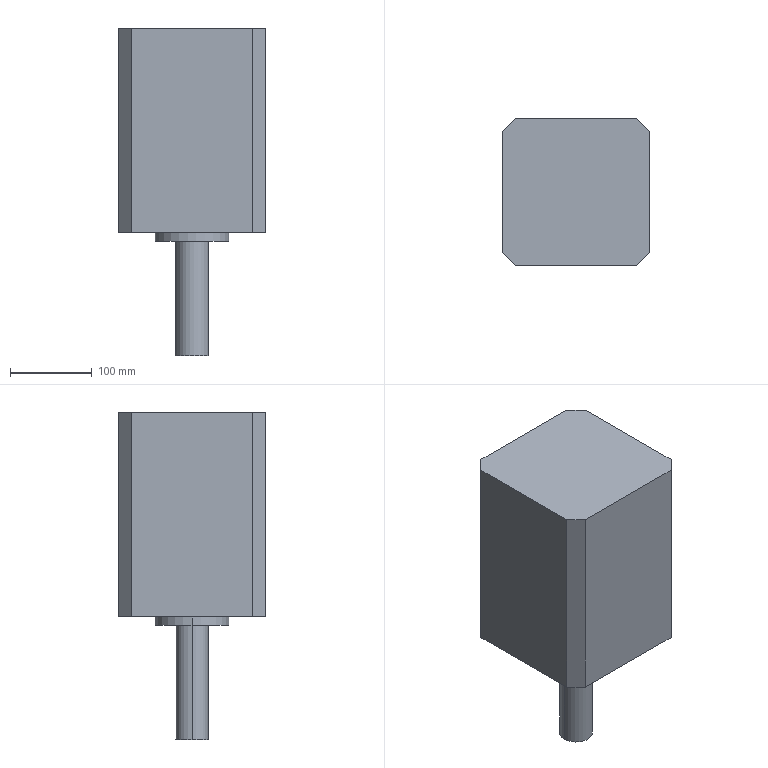Part | SolidWorks | features ICE 2, Chamfer 1, Extrusion 1 | 1 solid | 16 faces | box 180 x 180 x 400 mm | volume 8211546 mm3 | plane 12 | cylinder 4 | commonest cylinder face diameters 40 x2 90 x2
STEP:
#1=CARTESIAN_POINT('',(45.,0.,150.));
#2=VERTEX_POINT('',#1);
#3=CARTESIAN_POINT('',(-45.,0.,150.));
#4=VERTEX_POINT('',#3);
#5=CARTESIAN_POINT('',(0.,0.,150.));
#6=DIRECTION('',(0.,0.,1.));
#7=DIRECTION('',(1.,0.,0.));
#8=AXIS2_PLACEMENT_3D('',#5,#6,#7);
#9=CIRCLE('',#8,45.);
#10=EDGE_CURVE('',#2,#4,#9,.T.);
#11=ORIENTED_EDGE('',*,*,#10,.F.);
#12=CARTESIAN_POINT('',(45.,0.,140.));
#13=VERTEX_POINT('',#12);
#14=CARTESIAN_POINT('',(45.,0.,150.));
#15=DIRECTION('',(0.,0.,-1.));
#16=VECTOR('',#15,1000.);
#17=LINE('',#14,#16);
#18=EDGE_CURVE('',#2,#13,#17,.T.);
#19=ORIENTED_EDGE('',*,*,#18,.T.);
#20=CARTESIAN_POINT('',(-45.,0.,140.));
#21=VERTEX_POINT('',#20);
#22=CARTESIAN_POINT('',(0.,0.,140.));
#23=DIRECTION('',(0.,0.,1.));
#24=DIRECTION('',(1.,0.,0.));
#25=AXIS2_PLACEMENT_3D('',#22,#23,#24);
#26=CIRCLE('',#25,45.);
#27=EDGE_CURVE('',#13,#21,#26,.T.);
#28=ORIENTED_EDGE('',*,*,#27,.T.);
#29=CARTESIAN_POINT('',(-45.,0.,150.));
#30=DIRECTION('',(0.,0.,-1.));
#31=VECTOR('',#30,1000.);
#32=LINE('',#29,#31);
#33=EDGE_CURVE('',#4,#21,#32,.T.);
#34=ORIENTED_EDGE('',*,*,#33,.F.);
#35=EDGE_LOOP('',(#11,#19,#28,#34));
#36=FACE_OUTER_BOUND('',#35,.T.);
#37=CARTESIAN_POINT('',(0.,0.,150.));
#38=DIRECTION('',(0.,0.,-1.));
#39=DIRECTION('',(-1.,0.,0.));
#40=AXIS2_PLACEMENT_3D('',#37,#38,#39);
#41=CYLINDRICAL_SURFACE('',#40,45.);
#42=ADVANCED_FACE('',(#36),#41,.T.);
#43=CARTESIAN_POINT('',(20.,0.,140.));
#44=VERTEX_POINT('',#43);
#45=CARTESIAN_POINT('',(-20.,0.,140.));
#46=VERTEX_POINT('',#45);
#47=CARTESIAN_POINT('',(0.,0.,140.));
#48=DIRECTION('',(0.,0.,1.));
#49=DIRECTION('',(1.,0.,0.));
#50=AXIS2_PLACEMENT_3D('',#47,#48,#49);
#51=CIRCLE('',#50,20.);
#52=EDGE_CURVE('',#44,#46,#51,.T.);
#53=ORIENTED_EDGE('',*,*,#52,.F.);
#54=CARTESIAN_POINT('',(20.,0.,0.));
#55=VERTEX_POINT('',#54);
#56=CARTESIAN_POINT('',(20.,0.,140.));
#57=DIRECTION('',(0.,0.,-1.));
#58=VECTOR('',#57,1000.);
#59=LINE('',#56,#58);
#60=EDGE_CURVE('',#44,#55,#59,.T.);
#61=ORIENTED_EDGE('',*,*,#60,.T.);
#62=CARTESIAN_POINT('',(-20.,0.,0.));
#63=VERTEX_POINT('',#62);
#64=CARTESIAN_POINT('',(0.,0.,0.));
#65=DIRECTION('',(0.,0.,1.));
#66=DIRECTION('',(1.,0.,0.));
#67=AXIS2_PLACEMENT_3D('',#64,#65,#66);
#68=CIRCLE('',#67,20.);
#69=EDGE_CURVE('',#55,#63,#68,.T.);
#70=ORIENTED_EDGE('',*,*,#69,.T.);
#71=CARTESIAN_POINT('',(-20.,0.,140.));
#72=DIRECTION('',(0.,0.,-1.));
#73=VECTOR('',#72,1000.);
#74=LINE('',#71,#73);
#75=EDGE_CURVE('',#46,#63,#74,.T.);
#76=ORIENTED_EDGE('',*,*,#75,.F.);
#77=EDGE_LOOP('',(#53,#61,#70,#76));
#78=FACE_OUTER_BOUND('',#77,.T.);
#79=CARTESIAN_POINT('',(0.,0.,140.));
#80=DIRECTION('',(0.,0.,-1.));
#81=DIRECTION('',(-1.,0.,0.));
#82=AXIS2_PLACEMENT_3D('',#79,#80,#81);
#83=CYLINDRICAL_SURFACE('',#82,20.);
#84=ADVANCED_FACE('',(#78),#83,.T.);
#85=ORIENTED_EDGE('',*,*,#60,.F.);
#86=CARTESIAN_POINT('',(0.,0.,140.));
#87=DIRECTION('',(0.,0.,1.));
#88=DIRECTION('',(1.,0.,0.));
#89=AXIS2_PLACEMENT_3D('',#86,#87,#88);
#90=CIRCLE('',#89,20.);
#91=EDGE_CURVE('',#46,#44,#90,.T.);
#92=ORIENTED_EDGE('',*,*,#91,.F.);
#93=ORIENTED_EDGE('',*,*,#75,.T.);
#94=CARTESIAN_POINT('',(0.,0.,0.));
#95=DIRECTION('',(0.,0.,1.));
#96=DIRECTION('',(1.,0.,0.));
#97=AXIS2_PLACEMENT_3D('',#94,#95,#96);
#98=CIRCLE('',#97,20.);
#99=EDGE_CURVE('',#63,#55,#98,.T.);
#100=ORIENTED_EDGE('',*,*,#99,.T.);
#101=EDGE_LOOP('',(#85,#92,#93,#100));
#102=FACE_OUTER_BOUND('',#101,.T.);
#103=CARTESIAN_POINT('',(0.,0.,140.));
#104=DIRECTION('',(0.,0.,-1.));
#105=DIRECTION('',(-1.,0.,0.));
#106=AXIS2_PLACEMENT_3D('',#103,#104,#105);
#107=CYLINDRICAL_SURFACE('',#106,20.);
#108=ADVANCED_FACE('',(#102),#107,.T.);
#109=ORIENTED_EDGE('',*,*,#99,.F.);
#110=ORIENTED_EDGE('',*,*,#69,.F.);
#111=EDGE_LOOP('',(#109,#110));
#112=FACE_OUTER_BOUND('',#111,.T.);
#113=CARTESIAN_POINT('',(0.,0.,0.));
#114=DIRECTION('',(0.,0.,1.));
#115=DIRECTION('',(1.,0.,0.));
#116=AXIS2_PLACEMENT_3D('',#113,#114,#115);
#117=PLANE('',#116);
#118=ADVANCED_FACE('',(#112),#117,.F.);
#119=ORIENTED_EDGE('',*,*,#18,.F.);
#120=CARTESIAN_POINT('',(0.,0.,150.));
#121=DIRECTION('',(0.,0.,1.));
#122=DIRECTION('',(1.,0.,0.));
#123=AXIS2_PLACEMENT_3D('',#120,#121,#122);
#124=CIRCLE('',#123,45.);
#125=EDGE_CURVE('',#4,#2,#124,.T.);
#126=ORIENTED_EDGE('',*,*,#125,.F.);
#127=ORIENTED_EDGE('',*,*,#33,.T.);
#128=CARTESIAN_POINT('',(0.,0.,140.));
#129=DIRECTION('',(0.,0.,1.));
#130=DIRECTION('',(1.,0.,0.));
#131=AXIS2_PLACEMENT_3D('',#128,#129,#130);
#132=CIRCLE('',#131,45.);
#133=EDGE_CURVE('',#21,#13,#132,.T.);
#134=ORIENTED_EDGE('',*,*,#133,.T.);
#135=EDGE_LOOP('',(#119,#126,#127,#134));
#136=FACE_OUTER_BOUND('',#135,.T.);
#137=CARTESIAN_POINT('',(0.,0.,150.));
#138=DIRECTION('',(0.,0.,-1.));
#139=DIRECTION('',(-1.,0.,0.));
#140=AXIS2_PLACEMENT_3D('',#137,#138,#139);
#141=CYLINDRICAL_SURFACE('',#140,45.);
#142=ADVANCED_FACE('',(#136),#141,.T.);
#143=ORIENTED_EDGE('',*,*,#91,.T.);
#144=ORIENTED_EDGE('',*,*,#52,.T.);
#145=EDGE_LOOP('',(#143,#144));
#146=FACE_BOUND('',#145,.T.);
#147=ORIENTED_EDGE('',*,*,#133,.F.);
#148=ORIENTED_EDGE('',*,*,#27,.F.);
#149=EDGE_LOOP('',(#147,#148));
#150=FACE_OUTER_BOUND('',#149,.T.);
#151=CARTESIAN_POINT('',(0.,0.,140.));
#152=DIRECTION('',(0.,0.,1.));
#153=DIRECTION('',(1.,0.,0.));
#154=AXIS2_PLACEMENT_3D('',#151,#152,#153);
#155=PLANE('',#154);
#156=ADVANCED_FACE('',(#146,#150),#155,.F.);
#157=CARTESIAN_POINT('',(90.,-74.,400.));
#158=VERTEX_POINT('',#157);
#159=CARTESIAN_POINT('',(90.,74.,400.));
#160=VERTEX_POINT('',#159);
#161=CARTESIAN_POINT('',(90.,90.,400.));
#162=DIRECTION('',(0.,1.,0.));
#163=VECTOR('',#162,1000.);
#164=LINE('',#161,#163);
#165=EDGE_CURVE('',#158,#160,#164,.T.);
#166=ORIENTED_EDGE('',*,*,#165,.F.);
#167=CARTESIAN_POINT('',(90.,-74.,150.));
#168=VERTEX_POINT('',#167);
#169=CARTESIAN_POINT('',(90.,-74.,400.));
#170=DIRECTION('',(0.,0.,-1.));
#171=VECTOR('',#170,1000.);
#172=LINE('',#169,#171);
#173=EDGE_CURVE('',#158,#168,#172,.T.);
#174=ORIENTED_EDGE('',*,*,#173,.T.);
#175=CARTESIAN_POINT('',(90.,74.,150.));
#176=VERTEX_POINT('',#175);
#177=CARTESIAN_POINT('',(90.,90.,150.));
#178=DIRECTION('',(0.,1.,0.));
#179=VECTOR('',#178,1000.);
#180=LINE('',#177,#179);
#181=EDGE_CURVE('',#168,#176,#180,.T.);
#182=ORIENTED_EDGE('',*,*,#181,.T.);
#183=CARTESIAN_POINT('',(90.,74.,400.));
#184=DIRECTION('',(0.,0.,1.));
#185=VECTOR('',#184,1000.);
#186=LINE('',#183,#185);
#187=EDGE_CURVE('',#176,#160,#186,.T.);
#188=ORIENTED_EDGE('',*,*,#187,.T.);
#189=EDGE_LOOP('',(#166,#174,#182,#188));
#190=FACE_OUTER_BOUND('',#189,.T.);
#191=CARTESIAN_POINT('',(90.,90.,400.));
#192=DIRECTION('',(-1.,0.,0.));
#193=DIRECTION('',(0.,-1.,0.));
#194=AXIS2_PLACEMENT_3D('',#191,#192,#193);
#195=PLANE('',#194);
#196=ADVANCED_FACE('',(#190),#195,.F.);
#197=CARTESIAN_POINT('',(74.,90.,150.));
#198=VERTEX_POINT('',#197);
#199=CARTESIAN_POINT('',(-74.,90.,150.));
#200=VERTEX_POINT('',#199);
#201=CARTESIAN_POINT('',(-90.,90.,150.));
#202=DIRECTION('',(-1.,0.,0.));
#203=VECTOR('',#202,1000.);
#204=LINE('',#201,#203);
#205=EDGE_CURVE('',#198,#200,#204,.T.);
#206=ORIENTED_EDGE('',*,*,#205,.T.);
#207=CARTESIAN_POINT('',(-74.,90.,400.));
#208=VERTEX_POINT('',#207);
#209=CARTESIAN_POINT('',(-74.,90.,400.));
#210=DIRECTION('',(0.,0.,1.));
#211=VECTOR('',#210,1000.);
#212=LINE('',#209,#211);
#213=EDGE_CURVE('',#200,#208,#212,.T.);
#214=ORIENTED_EDGE('',*,*,#213,.T.);
#215=CARTESIAN_POINT('',(74.,90.,400.));
#216=VERTEX_POINT('',#215);
#217=CARTESIAN_POINT('',(-90.,90.,400.));
#218=DIRECTION('',(-1.,0.,0.));
#219=VECTOR('',#218,1000.);
#220=LINE('',#217,#219);
#221=EDGE_CURVE('',#216,#208,#220,.T.);
#222=ORIENTED_EDGE('',*,*,#221,.F.);
#223=CARTESIAN_POINT('',(74.,90.,400.));
#224=DIRECTION('',(0.,0.,-1.));
#225=VECTOR('',#224,1000.);
#226=LINE('',#223,#225);
#227=EDGE_CURVE('',#216,#198,#226,.T.);
#228=ORIENTED_EDGE('',*,*,#227,.T.);
#229=EDGE_LOOP('',(#206,#214,#222,#228));
#230=FACE_OUTER_BOUND('',#229,.T.);
#231=CARTESIAN_POINT('',(-90.,90.,400.));
#232=DIRECTION('',(0.,-1.,0.));
#233=DIRECTION('',(0.,0.,-1.));
#234=AXIS2_PLACEMENT_3D('',#231,#232,#233);
#235=PLANE('',#234);
#236=ADVANCED_FACE('',(#230),#235,.F.);
#237=CARTESIAN_POINT('',(-90.,74.,150.));
#238=VERTEX_POINT('',#237);
#239=CARTESIAN_POINT('',(-90.,-74.,150.));
#240=VERTEX_POINT('',#239);
#241=CARTESIAN_POINT('',(-90.,90.,150.));
#242=DIRECTION('',(0.,-1.,0.));
#243=VECTOR('',#242,1000.);
#244=LINE('',#241,#243);
#245=EDGE_CURVE('',#238,#240,#244,.T.);
#246=ORIENTED_EDGE('',*,*,#245,.T.);
#247=CARTESIAN_POINT('',(-90.,-74.,400.));
#248=VERTEX_POINT('',#247);
#249=CARTESIAN_POINT('',(-90.,-74.,400.));
#250=DIRECTION('',(0.,0.,1.));
#251=VECTOR('',#250,1000.);
#252=LINE('',#249,#251);
#253=EDGE_CURVE('',#240,#248,#252,.T.);
#254=ORIENTED_EDGE('',*,*,#253,.T.);
#255=CARTESIAN_POINT('',(-90.,74.,400.));
#256=VERTEX_POINT('',#255);
#257=CARTESIAN_POINT('',(-90.,90.,400.));
#258=DIRECTION('',(0.,-1.,0.));
#259=VECTOR('',#258,1000.);
#260=LINE('',#257,#259);
#261=EDGE_CURVE('',#256,#248,#260,.T.);
#262=ORIENTED_EDGE('',*,*,#261,.F.);
#263=CARTESIAN_POINT('',(-90.,74.,400.));
#264=DIRECTION('',(0.,0.,-1.));
#265=VECTOR('',#264,1000.);
#266=LINE('',#263,#265);
#267=EDGE_CURVE('',#256,#238,#266,.T.);
#268=ORIENTED_EDGE('',*,*,#267,.T.);
#269=EDGE_LOOP('',(#246,#254,#262,#268));
#270=FACE_OUTER_BOUND('',#269,.T.);
#271=CARTESIAN_POINT('',(-90.,90.,400.));
#272=DIRECTION('',(1.,0.,0.));
#273=DIRECTION('',(0.,1.,0.));
#274=AXIS2_PLACEMENT_3D('',#271,#272,#273);
#275=PLANE('',#274);
#276=ADVANCED_FACE('',(#270),#275,.F.);
#277=CARTESIAN_POINT('',(-74.,-90.,150.));
#278=VERTEX_POINT('',#277);
#279=CARTESIAN_POINT('',(74.,-90.,150.));
#280=VERTEX_POINT('',#279);
#281=CARTESIAN_POINT('',(-90.,-90.,150.));
#282=DIRECTION('',(1.,0.,0.));
#283=VECTOR('',#282,1000.);
#284=LINE('',#281,#283);
#285=EDGE_CURVE('',#278,#280,#284,.T.);
#286=ORIENTED_EDGE('',*,*,#285,.T.);
#287=CARTESIAN_POINT('',(74.,-90.,400.));
#288=VERTEX_POINT('',#287);
#289=CARTESIAN_POINT('',(74.,-90.,400.));
#290=DIRECTION('',(0.,0.,1.));
#291=VECTOR('',#290,1000.);
#292=LINE('',#289,#291);
#293=EDGE_CURVE('',#280,#288,#292,.T.);
#294=ORIENTED_EDGE('',*,*,#293,.T.);
#295=CARTESIAN_POINT('',(-74.,-90.,400.));
#296=VERTEX_POINT('',#295);
#297=CARTESIAN_POINT('',(-90.,-90.,400.));
#298=DIRECTION('',(1.,0.,0.));
#299=VECTOR('',#298,1000.);
#300=LINE('',#297,#299);
#301=EDGE_CURVE('',#296,#288,#300,.T.);
#302=ORIENTED_EDGE('',*,*,#301,.F.);
#303=CARTESIAN_POINT('',(-74.,-90.,400.));
#304=DIRECTION('',(0.,0.,-1.));
#305=VECTOR('',#304,1000.);
#306=LINE('',#303,#305);
#307=EDGE_CURVE('',#296,#278,#306,.T.);
#308=ORIENTED_EDGE('',*,*,#307,.T.);
#309=EDGE_LOOP('',(#286,#294,#302,#308));
#310=FACE_OUTER_BOUND('',#309,.T.);
#311=CARTESIAN_POINT('',(-90.,-90.,400.));
#312=DIRECTION('',(0.,1.,0.));
#313=DIRECTION('',(0.,0.,1.));
#314=AXIS2_PLACEMENT_3D('',#311,#312,#313);
#315=PLANE('',#314);
#316=ADVANCED_FACE('',(#310),#315,.F.);
#317=ORIENTED_EDGE('',*,*,#301,.T.);
#318=CARTESIAN_POINT('',(82.,-82.,400.));
#319=DIRECTION('',(0.7071,0.7071,0.));
#320=VECTOR('',#319,1000.);
#321=LINE('',#318,#320);
#322=EDGE_CURVE('',#288,#158,#321,.T.);
#323=ORIENTED_EDGE('',*,*,#322,.T.);
#324=ORIENTED_EDGE('',*,*,#165,.T.);
#325=CARTESIAN_POINT('',(82.,82.,400.));
#326=DIRECTION('',(-0.7071,0.7071,0.));
#327=VECTOR('',#326,1000.);
#328=LINE('',#325,#327);
#329=EDGE_CURVE('',#160,#216,#328,.T.);
#330=ORIENTED_EDGE('',*,*,#329,.T.);
#331=ORIENTED_EDGE('',*,*,#221,.T.);
#332=CARTESIAN_POINT('',(-82.,82.,400.));
#333=DIRECTION('',(-0.7071,-0.7071,0.));
#334=VECTOR('',#333,1000.);
#335=LINE('',#332,#334);
#336=EDGE_CURVE('',#208,#256,#335,.T.);
#337=ORIENTED_EDGE('',*,*,#336,.T.);
#338=ORIENTED_EDGE('',*,*,#261,.T.);
#339=CARTESIAN_POINT('',(-82.,-82.,400.));
#340=DIRECTION('',(0.7071,-0.7071,0.));
#341=VECTOR('',#340,1000.);
#342=LINE('',#339,#341);
#343=EDGE_CURVE('',#248,#296,#342,.T.);
#344=ORIENTED_EDGE('',*,*,#343,.T.);
#345=EDGE_LOOP('',(#317,#323,#324,#330,#331,#337,#338,#344));
#346=FACE_OUTER_BOUND('',#345,.T.);
#347=CARTESIAN_POINT('',(0.,0.,400.));
#348=DIRECTION('',(0.,0.,1.));
#349=DIRECTION('',(1.,0.,0.));
#350=AXIS2_PLACEMENT_3D('',#347,#348,#349);
#351=PLANE('',#350);
#352=ADVANCED_FACE('',(#346),#351,.T.);
#353=ORIENTED_EDGE('',*,*,#125,.T.);
#354=ORIENTED_EDGE('',*,*,#10,.T.);
#355=EDGE_LOOP('',(#353,#354));
#356=FACE_BOUND('',#355,.T.);
#357=ORIENTED_EDGE('',*,*,#181,.F.);
#358=CARTESIAN_POINT('',(90.,-74.,150.));
#359=DIRECTION('',(-0.7071,-0.7071,0.));
#360=VECTOR('',#359,1000.);
#361=LINE('',#358,#360);
#362=EDGE_CURVE('',#168,#280,#361,.T.);
#363=ORIENTED_EDGE('',*,*,#362,.T.);
#364=ORIENTED_EDGE('',*,*,#285,.F.);
#365=CARTESIAN_POINT('',(-74.,-90.,150.));
#366=DIRECTION('',(-0.7071,0.7071,0.));
#367=VECTOR('',#366,1000.);
#368=LINE('',#365,#367);
#369=EDGE_CURVE('',#278,#240,#368,.T.);
#370=ORIENTED_EDGE('',*,*,#369,.T.);
#371=ORIENTED_EDGE('',*,*,#245,.F.);
#372=CARTESIAN_POINT('',(-90.,74.,150.));
#373=DIRECTION('',(0.7071,0.7071,0.));
#374=VECTOR('',#373,1000.);
#375=LINE('',#372,#374);
#376=EDGE_CURVE('',#238,#200,#375,.T.);
#377=ORIENTED_EDGE('',*,*,#376,.T.);
#378=ORIENTED_EDGE('',*,*,#205,.F.);
#379=CARTESIAN_POINT('',(74.,90.,150.));
#380=DIRECTION('',(0.7071,-0.7071,0.));
#381=VECTOR('',#380,1000.);
#382=LINE('',#379,#381);
#383=EDGE_CURVE('',#198,#176,#382,.T.);
#384=ORIENTED_EDGE('',*,*,#383,.T.);
#385=EDGE_LOOP('',(#357,#363,#364,#370,#371,#377,#378,#384));
#386=FACE_OUTER_BOUND('',#385,.T.);
#387=CARTESIAN_POINT('',(0.,0.,150.));
#388=DIRECTION('',(0.,0.,1.));
#389=DIRECTION('',(1.,0.,0.));
#390=AXIS2_PLACEMENT_3D('',#387,#388,#389);
#391=PLANE('',#390);
#392=ADVANCED_FACE('',(#356,#386),#391,.F.);
#393=ORIENTED_EDGE('',*,*,#322,.F.);
#394=ORIENTED_EDGE('',*,*,#293,.F.);
#395=ORIENTED_EDGE('',*,*,#362,.F.);
#396=ORIENTED_EDGE('',*,*,#173,.F.);
#397=EDGE_LOOP('',(#393,#394,#395,#396));
#398=FACE_OUTER_BOUND('',#397,.T.);
#399=CARTESIAN_POINT('',(90.,-74.,400.));
#400=DIRECTION('',(-0.7071,0.7071,0.));
#401=DIRECTION('',(0.,0.,-1.));
#402=AXIS2_PLACEMENT_3D('',#399,#400,#401);
#403=PLANE('',#402);
#404=ADVANCED_FACE('',(#398),#403,.F.);
#405=ORIENTED_EDGE('',*,*,#343,.F.);
#406=ORIENTED_EDGE('',*,*,#253,.F.);
#407=ORIENTED_EDGE('',*,*,#369,.F.);
#408=ORIENTED_EDGE('',*,*,#307,.F.);
#409=EDGE_LOOP('',(#405,#406,#407,#408));
#410=FACE_OUTER_BOUND('',#409,.T.);
#411=CARTESIAN_POINT('',(-74.,-90.,400.));
#412=DIRECTION('',(0.7071,0.7071,0.));
#413=DIRECTION('',(0.,0.,-1.));
#414=AXIS2_PLACEMENT_3D('',#411,#412,#413);
#415=PLANE('',#414);
#416=ADVANCED_FACE('',(#410),#415,.F.);
#417=ORIENTED_EDGE('',*,*,#336,.F.);
#418=ORIENTED_EDGE('',*,*,#213,.F.);
#419=ORIENTED_EDGE('',*,*,#376,.F.);
#420=ORIENTED_EDGE('',*,*,#267,.F.);
#421=EDGE_LOOP('',(#417,#418,#419,#420));
#422=FACE_OUTER_BOUND('',#421,.T.);
#423=CARTESIAN_POINT('',(-90.,74.,400.));
#424=DIRECTION('',(0.7071,-0.7071,0.));
#425=DIRECTION('',(0.,0.,-1.));
#426=AXIS2_PLACEMENT_3D('',#423,#424,#425);
#427=PLANE('',#426);
#428=ADVANCED_FACE('',(#422),#427,.F.);
#429=ORIENTED_EDGE('',*,*,#329,.F.);
#430=ORIENTED_EDGE('',*,*,#187,.F.);
#431=ORIENTED_EDGE('',*,*,#383,.F.);
#432=ORIENTED_EDGE('',*,*,#227,.F.);
#433=EDGE_LOOP('',(#429,#430,#431,#432));
#434=FACE_OUTER_BOUND('',#433,.T.);
#435=CARTESIAN_POINT('',(74.,90.,400.));
#436=DIRECTION('',(-0.7071,-0.7071,0.));
#437=DIRECTION('',(0.,0.,-1.));
#438=AXIS2_PLACEMENT_3D('',#435,#436,#437);
#439=PLANE('',#438);
#440=ADVANCED_FACE('',(#434),#439,.F.);
#441=CLOSED_SHELL('',(#42,#84,#108,#118,#142,#156,#196,#236,#276,#316,#352,#392,#404,#416,#428,#440));
#442=MANIFOLD_SOLID_BREP('',#441);
#443=CARTESIAN_POINT('',(0.,0.,0.));
#444=DIRECTION('',(0.,0.,1.));
#445=DIRECTION('',(1.,0.,0.));
#446=AXIS2_PLACEMENT_3D('',#443,#444,#445);
#447=(LENGTH_UNIT()NAMED_UNIT(*)SI_UNIT(.MILLI.,.METRE.));
#448=UNCERTAINTY_MEASURE_WITH_UNIT(LENGTH_MEASURE(0.00001),#447,'','');
#449=(NAMED_UNIT(*)PLANE_ANGLE_UNIT()SI_UNIT($,.RADIAN.));
#450=(NAMED_UNIT(*)SI_UNIT($,.STERADIAN.)SOLID_ANGLE_UNIT());
#451=(GEOMETRIC_REPRESENTATION_CONTEXT(3)GLOBAL_UNCERTAINTY_ASSIGNED_CONTEXT((#448))GLOBAL_UNIT_ASSIGNED_CONTEXT((#447,#449,#450))REPRESENTATION_CONTEXT('',''));
#452=ADVANCED_BREP_SHAPE_REPRESENTATION('',(#442,#446),#451);